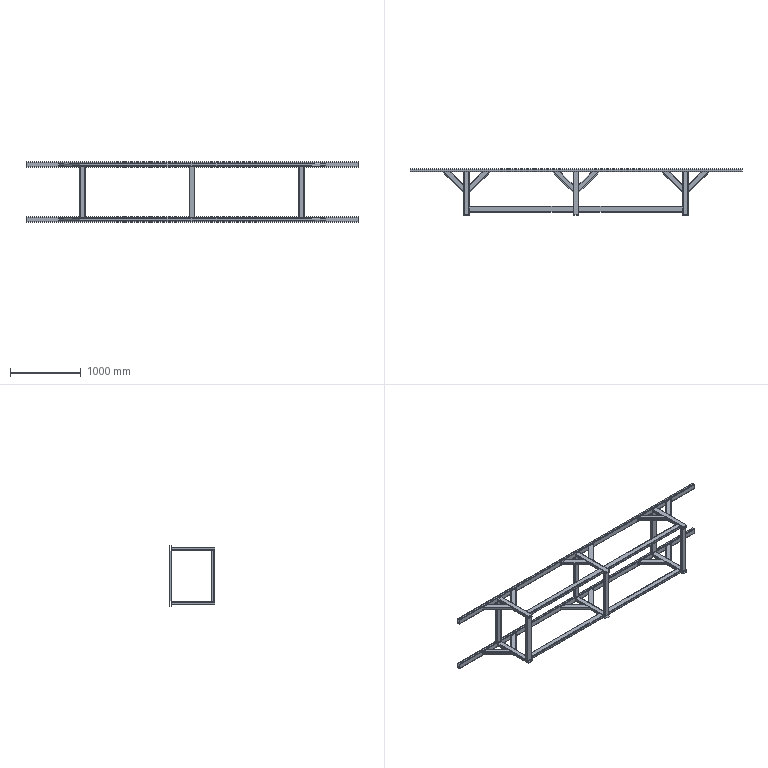Part | SolidWorks | features WeldCornerFeat 3, 3DProfileFeature 1, MoveCopyBody 1, WeldMemberFeat 1, WeldmentFeature 1 | 30 solids | 540 faces | box 4700 x 650 x 854 mm | volume 23333323 mm3 | plane 300 | cylinder 240 | commonest cylinder face diameters 8 x120 16 x120